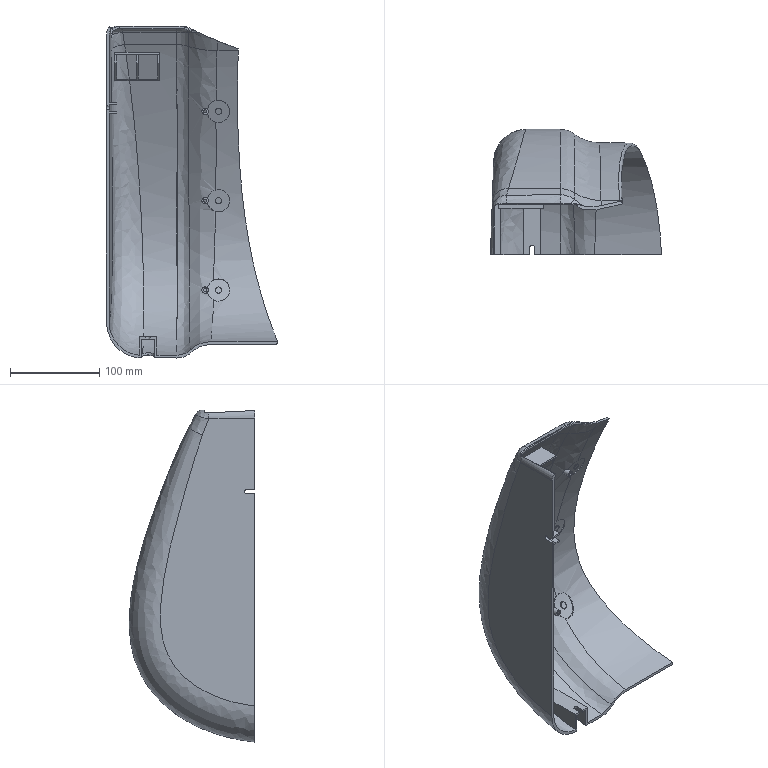Part | STEP file | MOTOR COVER L | 1 solid | 131 faces | box 191.608 x 140.54 x 371.606 mm | volume 339460 mm3 | spline 58 | plane 54 | cylinder 19 | commonest cylinder face diameters 7 x6 3.6 x3 25 x3 14 x2 16 x2 4 x1